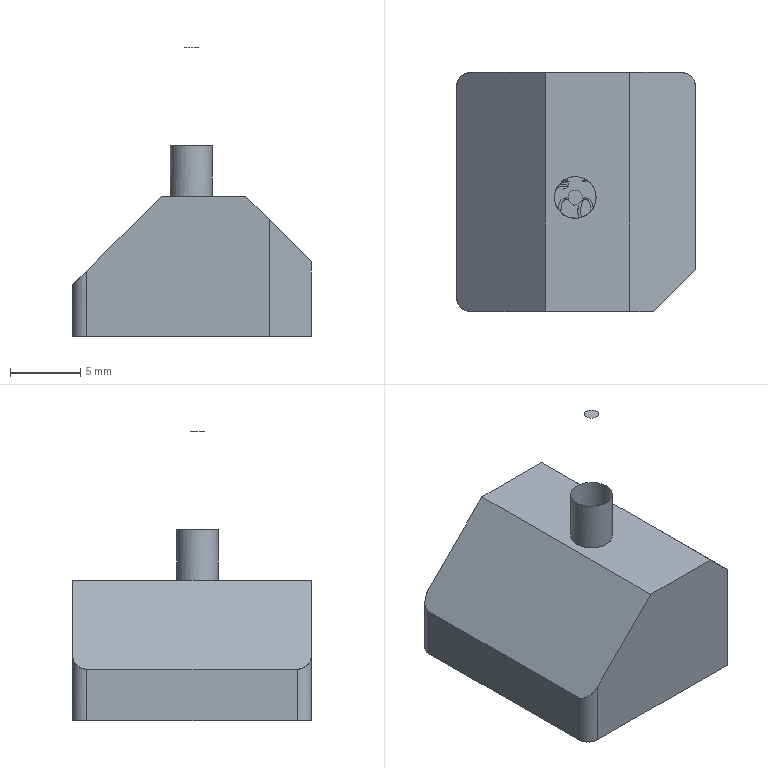NC program | PowerMill | posted with a generic post | part box 17 x 17 x 20.603 mm
Lines 1 to 1059 of 42778:
%
O0001
N104 ( POWERMILL CB  : 2026004.0)
N105 ( POST VER      : 2026.0.0.5161)
N106 ( OPTION FILE   : FANUC)
N107 ( OUTPUT WORKPLANE : WORLD)
N108 (  )
N109 ( TOOL LIST )
N110 (---------------------------------------)
N111 ( NO. | ID        | DIA.| TIP RAD|LENGTH)
N112 (---------------------------------------)
N113 (    1|D10C_1_1_1 |10.0 |  0.0   |76.04 )
N114 (    3|D10_1_1_1  |10.0 |  0.0   |75.76 )
N115 (   14|D4_2_1     | 4.0 |  0.0   |65.68 )
N116 (    7|R2_2_1     | 4.0 |  2.0   |73.16 )
N117 (   13|TEXT_D4_1_1| 4.0 |  0.3   |65.88 )
N118 (---------------------------------------)
N119 (  )
N120 ( NUMBER OF TOOLPATHS: 10.0 )
N121 ( ESTIMATED PROGRAM DURATION: 0 HOURS 5 MIN 41 SEC)
N122 (  )
N123 G00 G21 G80 G40 G17
N124 G90
N125 G54
N126 G53 Z0.0
N127 (---------------)
N128 ( START TOOLPATH : 粗公开粗01-扫面平行-D10C )
N129 (---------------)
N130 ( TOOL NO.    :1 )
N131 ( TOOL TYPE   : ENDMILL)
N132 ( TOOL ID     : D10C_1_1_1)
N133 ( TOOL DIA    : 10.0 LENGTH 76.04)
N134 T1
N135 M6
N136 S8000 M03
N137 G00 G90 X0.002 Y0.0
N138 G43 Z10.2 H1
N139
N140 G05 P10000 R4
N141 X16.202 Y11.2
N142 Z1.053
N143 G01 Z-0.147 F6000.0
N144 X11.202 F10000.0
N145 X-11.198
N146 Y5.6
N147 X11.202
N148 Y0.0
N149 X-11.198
N150 Y-5.6
N151 X11.202
N152 Y-11.2
N153 X-11.198
N154 X-16.198
N155 G00 Z10.2
N156 G05 P0
N157 (---------------)
N158 ( END TOOLPATH : 粗公开粗01-扫面平行-D10C )
N159 (---------------)
N160 ( START TOOLPATH : 粗公开粗01-外形偏置-D10C )
N161 (---------------)
N162 G00 X0.002 Y0.0 Z9.803
N163 G05 P10000 R4
N164 X5.2164 Y-16.475
N165 Z0.6159
N166 G01 Z-0.5841 F6000.0
N167 Y-15.9475 F10000.0
N168 G03 X0.4689 Y-11.2 I-4.7475 J0.0
N169 G01 X-10.198
N170 G02 X-11.198 Y-10.2 I0.0 J1.0
N171 G01 Y10.2
N172 G02 X-10.198 Y11.2 I1.0 J0.0
N173 G01 X10.202
N174 G02 X11.202 Y10.2 I0.0 J-1.0
N175 G01 Y-10.2
N176 G02 X10.202 Y-11.2 I-1.0 J0.0
N177 G01 X0.4689
N178 X0.3887 Y-6.1325
N179 X-0.3847 Y-6.1447
N180 X-1.1581 Y-6.0422
N181 X-1.9316 Y-5.8387
N182 X-2.705 Y-5.5007
N183 X-3.4724 Y-5.0273
N184 X-4.2518 Y-4.3313
N185 X-4.9075 Y-3.4804
N186 X-5.3237 Y-2.707
N187 X-5.5933 Y-1.9336
N188 X-5.7564 Y-1.1601
N189 X-5.8016 Y-0.3867
N190 X-5.7528 Y0.3867
N191 X-5.5859 Y1.1601
N192 X-5.3119 Y1.9336
N193 X-4.8907 Y2.707
N194 X-4.2993 Y3.4804
N195 X-3.4784 Y4.2225
N196 X-2.705 Y4.7005
N197 X-1.9645 Y5.0273
N198 X-1.1581 Y5.2423
N199 X-0.3847 Y5.3447
N200 X0.3887 Y5.3325
N201 X1.1621 Y5.2245
N202 X1.8447 Y5.0273
N203 X2.709 Y4.6479
N204 X3.4824 Y4.1366
N205 X4.1932 Y3.4804
N206 X4.7904 Y2.707
N207 X5.0293 Y2.2968
N208 X5.202 Y1.9336
N209 X5.4862 Y1.1601
N210 X5.6427 Y0.3867
N211 X5.702 Y-0.3867
N212 X5.6464 Y-1.1601
N213 X5.4936 Y-1.9336
N214 X5.2135 Y-2.707
N215 X5.0293 Y-3.0966
N216 X4.8073 Y-3.4804
N217 X4.2558 Y-4.2102
N218 X3.4824 Y-4.9368
N219 X2.709 Y-5.4482
N220 X1.9193 Y-5.8007
N221 X1.1621 Y-6.0245
N222 X0.3887 Y-6.1325
N223 X0.4689 Y-11.2
N224 G00 Z3.2287
N225 G01 X5.2164 Y-16.475
N226 G00 Z0.2287
N227 G01 Z-0.9713 F6000.0
N228 Y-15.9475 F10000.0
N229 G03 X0.4689 Y-11.2 I-4.7475 J0.0
N230 G01 X-10.198
N231 G02 X-11.198 Y-10.2 I0.0 J1.0
N232 G01 Y10.2
N233 G02 X-10.198 Y11.2 I1.0 J0.0
N234 G01 X10.202
N235 G02 X11.202 Y10.2 I0.0 J-1.0
N236 G01 Y-10.2
N237 G02 X10.202 Y-11.2 I-1.0 J0.0
N238 G01 X0.471
N239 X0.3887 Y-6.1865
N240 X-0.3847 Y-6.1992
N241 X-1.1581 Y-6.0972
N242 X-1.9316 Y-5.8961
N243 X-2.705 Y-5.5614
N244 X-3.4784 Y-5.0908
N245 X-4.2518 Y-4.4099
N246 X-4.3964 Y-4.2538
N247 X-4.9706 Y-3.4804
N248 X-5.3827 Y-2.707
N249 X-5.6493 Y-1.9336
N250 X-5.7987 Y-1.2475
N251 X-5.8555 Y-0.3867
N252 X-5.8077 Y0.3867
N253 X-5.6419 Y1.1601
N254 X-5.371 Y1.9336
N255 X-5.0253 Y2.5909
N256 X-4.3724 Y3.4804
N257 X-3.528 Y4.2538
N258 X-2.705 Y4.761
N259 X-2.1221 Y5.0273
N260 X-1.1581 Y5.2973
N261 X-0.3847 Y5.3992
N262 X0.3887 Y5.3865
N263 X1.1621 Y5.28
N264 X1.9356 Y5.0521
N265 X2.709 Y4.7095
N266 X3.4158 Y4.2538
N267 X4.2558 Y3.4915
N268 X4.8545 Y2.707
N269 X5.0293 Y2.4118
N270 X5.2607 Y1.9336
N271 X5.5424 Y1.1601
N272 X5.6972 Y0.3867
N273 X5.7564 Y-0.3867
N274 X5.7008 Y-1.1601
N275 X5.5498 Y-1.9336
N276 X5.2721 Y-2.707
N277 X5.0293 Y-3.2119
N278 X4.8713 Y-3.4804
N279 X4.2887 Y-4.2538
N280 X3.4824 Y-5.0044
N281 X2.709 Y-5.5102
N282 X2.0755 Y-5.8007
N283 X1.1621 Y-6.08
N284 X0.3887 Y-6.1865
N285 X0.471 Y-11.2
N286 X0.4689
N287 G00 Z2.8416
N288 G01 X5.2164 Y-16.475
N289 G00 Z-0.1584
N290 G01 Z-1.3584 F6000.0
N291 Y-15.9475 F10000.0
N292 G03 X0.4689 Y-11.2 I-4.7475 J0.0
N293 G01 X-10.198
N294 G02 X-11.198 Y-10.2 I0.0 J1.0
N295 G01 Y10.2
N296 G02 X-10.198 Y11.2 I1.0 J0.0
N297 G01 X10.202
N298 G02 X11.202 Y10.2 I0.0 J-1.0
N299 G01 Y-10.2
N300 G02 X10.202 Y-11.2 I-1.0 J0.0
N301 G01 X0.4729
N302 X0.3887 Y-6.2405
N303 X-0.3847 Y-6.2537
N304 X-1.1581 Y-6.1522
N305 X-1.9316 Y-5.9534
N306 X-2.3305 Y-5.8007
N307 X-2.705 Y-5.622
N308 X-3.4784 Y-5.1573
N309 X-4.2518 Y-4.4867
N310 X-4.4692 Y-4.2538
N311 X-5.0253 Y-3.4945
N312 X-5.4417 Y-2.707
N313 X-5.7052 Y-1.9336
N314 X-5.8661 Y-1.1601
N315 X-5.9094 Y-0.3867
N316 X-5.8626 Y0.3867
N317 X-5.6978 Y1.1601
N318 X-5.4302 Y1.9336
N319 X-5.0253 Y2.6939
N320 X-4.4456 Y3.4804
N321 X-4.2518 Y3.6874
N322 X-3.6168 Y4.2538
N323 X-2.705 Y4.8215
N324 X-2.2679 Y5.0273
N325 X-1.9316 Y5.1529
N326 X-1.1581 Y5.3523
N327 X-0.3847 Y5.4537
N328 X0.3887 Y5.4405
N329 X1.1621 Y5.3355
N330 X1.9356 Y5.1093
N331 X2.709 Y4.7711
N332 X3.5078 Y4.2538
N333 X4.2558 Y3.5736
N334 X4.9187 Y2.707
N335 X5.3193 Y1.9336
N336 X5.5987 Y1.1601
N337 X5.7516 Y0.3867
N338 X5.8108 Y-0.3867
N339 X5.7552 Y-1.1601
N340 X5.6059 Y-1.9336
N341 X5.3307 Y-2.707
N342 X4.9353 Y-3.4804
N343 X4.3605 Y-4.2538
N344 X3.5428 Y-5.0273
N345 X2.709 Y-5.5721
N346 X2.2229 Y-5.8007
N347 X1.9356 Y-5.9093
N348 X1.1621 Y-6.1355
N349 X0.3887 Y-6.2405
N350 X0.4729 Y-11.2
N351 X0.4689
N352 G00 Z2.4544
N353 G01 X5.2164 Y-16.475
N354 G00 Z-0.5456
N355 G01 Z-1.7456 F6000.0
N356 Y-15.9475 F10000.0
N357 G03 X0.4689 Y-11.2 I-4.7475 J0.0
N358 G01 X-10.198
N359 G02 X-11.198 Y-10.2 I0.0 J1.0
N360 G01 Y10.2
N361 G02 X-10.198 Y11.2 I1.0 J0.0
N362 G01 X10.202
N363 G02 X11.202 Y10.2 I0.0 J-1.0
N364 G01 Y-10.2
N365 G02 X10.202 Y-11.2 I-1.0 J0.0
N366 G01 X0.4748
N367 X0.3887 Y-6.2946
N368 X-0.3847 Y-6.3082
N369 X-1.1581 Y-6.2073
N370 X-1.9316 Y-6.0108
N371 X-2.705 Y-5.6827
N372 X-3.4784 Y-5.2239
N373 X-3.7387 Y-5.0273
N374 X-4.2518 Y-4.5626
N375 X-4.542 Y-4.2538
N376 X-5.0253 Y-3.5981
N377 X-5.5007 Y-2.707
N378 X-5.7612 Y-1.9336
N379 X-5.9209 Y-1.1601
N380 X-5.9633 Y-0.3867
N381 X-5.9174 Y0.3867
N382 X-5.7987 Y0.9956
N383 X-5.4893 Y1.9336
N384 X-5.0804 Y2.707
N385 X-4.5187 Y3.4804
N386 X-4.2518 Y3.7627
N387 X-3.7052 Y4.2538
N388 X-3.4784 Y4.4241
N389 X-2.705 Y4.882
N390 X-2.4058 Y5.0273
N391 X-1.9316 Y5.2101
N392 X-1.1581 Y5.4074
N393 X-0.3847 Y5.5082
N394 X0.3887 Y5.4946
N395 X1.1621 Y5.3909
N396 X1.9356 Y5.1665
N397 X2.3013 Y5.0273
N398 X2.709 Y4.8327
N399 X3.4824 Y4.3397
N400 X4.2558 Y3.6535
N401 X4.409 Y3.4804
N402 X4.9828 Y2.707
N403 X5.3779 Y1.9336
N404 X5.6549 Y1.1601
N405 X5.8027 Y0.4104
N406 X5.8652 Y-0.3867
N407 X5.8096 Y-1.1601
N408 X5.6621 Y-1.9336
N409 X5.3893 Y-2.707
N410 X5.0293 Y-3.4311
N411 X4.4315 Y-4.2538
N412 X4.2558 Y-4.4542
N413 X3.6311 Y-5.0273
N414 X2.709 Y-5.6333
N415 X2.3621 Y-5.8007
N416 X1.9356 Y-5.9665
N417 X1.1621 Y-6.1909
N418 X0.3887 Y-6.2946
N419 X0.4748 Y-11.2
N420 X0.4689
N421 G00 Z2.0673
N422 G01 X5.2164 Y-16.475
N423 G00 Z-0.9327
N424 G01 Z-2.1327 F6000.0
N425 Y-15.9475 F10000.0
N426 G03 X0.4689 Y-11.2 I-4.7475 J0.0
N427 G01 X-10.198
N428 G02 X-11.198 Y-10.2 I0.0 J1.0
N429 G01 Y10.2
N430 G02 X-10.198 Y11.2 I1.0 J0.0
N431 G01 X10.202
N432 G02 X11.202 Y10.2 I0.0 J-1.0
N433 G01 Y-10.2
N434 G02 X10.202 Y-11.2 I-1.0 J0.0
N435 G01 X0.4766
N436 X0.3887 Y-6.3486
N437 X-0.3847 Y-6.3626
N438 X-1.1581 Y-6.2623
N439 X-1.9316 Y-6.0682
N440 X-2.5905 Y-5.8007
N441 X-3.4784 Y-5.2904
N442 X-3.8234 Y-5.0273
N443 X-4.2518 Y-4.6386
N444 X-4.614 Y-4.2538
N445 X-5.0253 Y-3.6982
N446 X-5.16 Y-3.4804
N447 X-5.5597 Y-2.707
N448 X-5.7987 Y-1.9995
N449 X-5.9757 Y-1.1601
N450 X-6.0172 Y-0.3867
N451 X-5.9723 Y0.3867
N452 X-5.8098 Y1.1601
N453 X-5.5485 Y1.9336
N454 X-5.0253 Y2.8991
N455 X-4.5914 Y3.4804
N456 X-4.2518 Y3.838
N457 X-3.7915 Y4.2538
N458 X-3.4784 Y4.4913
N459 X-2.705 Y4.9424
N460 X-1.9316 Y5.2673
N461 X-1.1581 Y5.4624
N462 X-0.3847 Y5.5626
N463 X0.3887 Y5.5486
N464 X1.1621 Y5.4464
N465 X1.9356 Y5.2237
N466 X2.4369 Y5.0273
N467 X2.709 Y4.8943
N468 X3.4824 Y4.4056
N469 X3.6855 Y4.2538
N470 X4.2558 Y3.7327
N471 X4.4787 Y3.4804
N472 X5.0293 Y2.7365
N473 X5.4366 Y1.9336
N474 X5.7112 Y1.1601
N475 X5.8604 Y0.3867
N476 X5.9196 Y-0.3867
N477 X5.864 Y-1.1601
N478 X5.7182 Y-1.9336
N479 X5.4479 Y-2.707
N480 X5.0632 Y-3.4804
N481 X4.5011 Y-4.2538
N482 X4.2558 Y-4.5328
N483 X3.7194 Y-5.0273
N484 X3.4824 Y-5.2058
N485 X2.709 Y-5.6944
N486 X2.4942 Y-5.8007
N487 X1.9356 Y-6.0237
N488 X1.1621 Y-6.2464
N489 X0.3887 Y-6.3486
N490 X0.4766 Y-11.2
N491 X0.4689
N492 G00 Z1.6801
N493 G01 X5.2164 Y-16.475
N494 G00 Z-1.3199
N495 G01 Z-2.5199 F6000.0
N496 Y-15.9475 F10000.0
N497 G03 X0.4689 Y-11.2 I-4.7475 J0.0
N498 G01 X-10.198
N499 G02 X-11.198 Y-10.2 I0.0 J1.0
N500 G01 Y10.2
N501 G02 X-10.198 Y11.2 I1.0 J0.0
N502 G01 X10.202
N503 G02 X11.202 Y10.2 I0.0 J-1.0
N504 G01 Y-10.2
N505 G02 X10.202 Y-11.2 I-1.0 J0.0
N506 G01 X0.4784
N507 X0.3887 Y-6.4026
N508 X-0.3847 Y-6.4171
N509 X-1.1581 Y-6.3174
N510 X-1.9316 Y-6.1255
N511 X-2.705 Y-5.804
N512 X-3.4784 Y-5.357
N513 X-3.9081 Y-5.0273
N514 X-4.2518 Y-4.713
N515 X-4.6845 Y-4.2538
N516 X-5.0253 Y-3.7983
N517 X-5.2231 Y-3.4804
N518 X-5.6187 Y-2.707
N519 X-5.8731 Y-1.9336
N520 X-6.0305 Y-1.1601
N521 X-6.0711 Y-0.3867
N522 X-6.0271 Y0.3867
N523 X-5.8657 Y1.1601
N524 X-5.6076 Y1.9336
N525 X-5.2068 Y2.707
N526 X-5.0253 Y2.9972
N527 X-4.6623 Y3.4804
N528 X-4.2518 Y3.9134
N529 X-3.8762 Y4.2538
N530 X-3.4784 Y4.5573
N531 X-2.6589 Y5.0273
N532 X-1.9316 Y5.3245
N533 X-1.1581 Y5.5175
N534 X-0.3847 Y5.6171
N535 X0.3887 Y5.6026
N536 X1.1621 Y5.5019
N537 X1.9356 Y5.2809
N538 X2.5657 Y5.0273
N539 X3.4824 Y4.4716
N540 X3.7727 Y4.2538
N541 X4.2558 Y3.8119
N542 X4.5483 Y3.4804
N543 X5.0293 Y2.8384
N544 X5.4952 Y1.9336
N545 X5.7674 Y1.1601
N546 X5.9148 Y0.3867
N547 X5.974 Y-0.3867
N548 X5.9184 Y-1.1601
N549 X5.8027 Y-1.8233
N550 X5.5065 Y-2.707
N551 X5.1272 Y-3.4804
N552 X4.5706 Y-4.2538
N553 X4.2558 Y-4.6115
N554 X3.8053 Y-5.0273
N555 X3.4824 Y-5.2718
N556 X2.6205 Y-5.8007
N557 X1.9356 Y-6.0809
N558 X1.1621 Y-6.3019
N559 X0.3887 Y-6.4026
N560 X0.4784 Y-11.2
N561 X0.4689
N562 G00 Z1.293
N563 G01 X5.2164 Y-16.475
N564 G00 Z-1.707
N565 G01 Z-2.907 F6000.0
N566 Y-15.9475 F10000.0
N567 G03 X0.4689 Y-11.2 I-4.7475 J0.0
N568 G01 X-10.198
N569 G02 X-11.198 Y-10.2 I0.0 J1.0
N570 G01 Y10.2
N571 G02 X-10.198 Y11.2 I1.0 J0.0
N572 G01 X10.202
N573 G02 X11.202 Y10.2 I0.0 J-1.0
N574 G01 Y-10.2
N575 G02 X10.202 Y-11.2 I-1.0 J0.0
N576 G01 X0.4801
N577 X0.3887 Y-6.4567
N578 X-0.3847 Y-6.4716
N579 X-1.1581 Y-6.3724
N580 X-1.9316 Y-6.1827
N581 X-2.705 Y-5.8647
N582 X-3.4784 Y-5.4235
N583 X-3.9903 Y-5.0273
N584 X-4.2518 Y-4.7867
N585 X-4.7551 Y-4.2538
N586 X-5.0253 Y-3.8941
N587 X-5.2862 Y-3.4804
N588 X-5.6777 Y-2.707
N589 X-5.929 Y-1.9336
N590 X-6.0853 Y-1.1601
N591 X-6.1251 Y-0.3867
N592 X-6.0819 Y0.3867
N593 X-5.9217 Y1.1601
N594 X-5.6667 Y1.9336
N595 X-5.27 Y2.707
N596 X-5.0253 Y3.0951
N597 X-4.7331 Y3.4804
N598 X-4.2518 Y3.9871
N599 X-3.9604 Y4.2538
N600 X-3.4784 Y4.6227
N601 X-2.7775 Y5.0273
N602 X-1.9316 Y5.3817
N603 X-1.1581 Y5.5725
N604 X-0.3847 Y5.6716
N605 X0.3887 Y5.6567
N606 X1.1621 Y5.5574
N607 X1.9356 Y5.3381
N608 X2.709 Y5.0176
N609 X3.4824 Y4.5376
N610 X3.8582 Y4.2538
N611 X4.2558 Y3.8899
N612 X4.6179 Y3.4804
N613 X5.0293 Y2.9377
N614 X5.1743 Y2.707
N615 X5.5538 Y1.9336
N616 X5.8027 Y1.2403
N617 X5.9692 Y0.3867
N618 X6.0284 Y-0.3867
N619 X5.9729 Y-1.1601
N620 X5.8305 Y-1.9336
N621 X5.5651 Y-2.707
N622 X5.1897 Y-3.4804
N623 X5.0293 Y-3.738
N624 X4.6402 Y-4.2538
N625 X4.2558 Y-4.6901
N626 X3.8902 Y-5.0273
N627 X3.4824 Y-5.3378
N628 X2.742 Y-5.8007
N629 X1.9356 Y-6.1381
N630 X1.1621 Y-6.3573
N631 X0.3887 Y-6.4567
N632 X0.4801 Y-11.2
N633 X0.4689
N634 G00 Z0.9058
N635 G01 X5.2164 Y-16.475
N636 G00 Z-2.0942
N637 G01 Z-3.2942 F6000.0
N638 Y-15.9475 F10000.0
N639 G03 X0.4689 Y-11.2 I-4.7475 J0.0
N640 G01 X-10.198
N641 G02 X-11.198 Y-10.2 I0.0 J1.0
N642 G01 Y10.2
N643 G02 X-10.198 Y11.2 I1.0 J0.0
N644 G01 X10.202
N645 G02 X11.202 Y10.2 I0.0 J-1.0
N646 G01 Y-10.2
N647 G02 X10.202 Y-11.2 I-1.0 J0.0
N648 G01 X0.4818
N649 X0.3887 Y-6.5107
N650 X-0.3847 Y-6.526
N651 X-1.1581 Y-6.4275
N652 X-1.9316 Y-6.2394
N653 X-2.705 Y-5.9253
N654 X-3.4784 Y-5.4887
N655 X-4.0717 Y-5.0273
N656 X-4.8256 Y-4.2538
N657 X-5.0253 Y-3.9899
N658 X-5.3493 Y-3.4804
N659 X-5.7367 Y-2.707
N660 X-5.985 Y-1.9336
N661 X-6.14 Y-1.1601
N662 X-6.179 Y-0.3867
N663 X-6.1367 Y0.3867
N664 X-5.9777 Y1.1601
N665 X-5.7259 Y1.9336
N666 X-5.3332 Y2.707
N667 X-5.0253 Y3.1891
N668 X-4.8039 Y3.4804
N669 X-4.0418 Y4.2538
N670 X-3.4784 Y4.6881
N671 X-2.8948 Y5.0273
N672 X-1.9316 Y5.4389
N673 X-1.1581 Y5.6275
N674 X-0.3847 Y5.726
N675 X0.3887 Y5.7107
N676 X1.1621 Y5.6128
N677 X1.9356 Y5.3953
N678 X2.709 Y5.0782
N679 X3.4824 Y4.6035
N680 X3.9437 Y4.2538
N681 X4.2558 Y3.9665
N682 X4.6876 Y3.4804
N683 X5.0293 Y3.035
N684 X5.2369 Y2.707
N685 X5.6125 Y1.9336
N686 X5.8027 Y1.4305
N687 X5.8799 Y1.1601
N688 X6.0236 Y0.3867
N689 X6.0828 Y-0.3867
N690 X6.0273 Y-1.1601
N691 X5.8867 Y-1.9336
N692 X5.8027 Y-2.231
N693 X5.6237 Y-2.707
N694 X5.2522 Y-3.4804
N695 X5.0293 Y-3.8347
N696 X4.7097 Y-4.2538
N697 X4.2558 Y-4.7668
N698 X3.9751 Y-5.0273
N699 X3.4824 Y-5.4038
N700 X2.8575 Y-5.8007
N701 X1.9356 Y-6.1953
N702 X1.1621 Y-6.4128
N703 X0.3887 Y-6.5107
N704 X0.4818 Y-11.2
N705 X0.4689
N706 G00 Z0.5187
N707 G01 X5.2164 Y-16.475
N708 G00 Z-2.4813
N709 G01 Z-3.6813 F6000.0
N710 Y-15.9475 F10000.0
N711 G03 X0.4689 Y-11.2 I-4.7475 J0.0
N712 G01 X-10.198
N713 G02 X-11.198 Y-10.2 I0.0 J1.0
N714 G01 Y10.2
N715 G02 X-10.198 Y11.2 I1.0 J0.0
N716 G01 X10.202
N717 G02 X11.202 Y10.2 I0.0 J-1.0
N718 G01 Y-10.2
N719 G02 X10.202 Y-11.2 I-1.0 J0.0
N720 G01 X0.7886
N721 X0.2512 Y-6.5741
N722 X-0.3847 Y-6.5805
N723 X-1.1581 Y-6.4825
N724 X-1.9316 Y-6.2961
N725 X-2.705 Y-5.9853
N726 X-3.4784 Y-5.5535
N727 X-4.1525 Y-5.0273
N728 X-4.8957 Y-4.2538
N729 X-5.4124 Y-3.4804
N730 X-5.7955 Y-2.707
N731 X-6.0409 Y-1.9336
N732 X-6.1948 Y-1.1601
N733 X-6.2329 Y-0.3867
N734 X-6.1915 Y0.3867
N735 X-6.0336 Y1.1601
N736 X-5.785 Y1.9336
N737 X-5.3964 Y2.707
N738 X-4.8746 Y3.4804
N739 X-4.2518 Y4.1346
N740 X-3.4784 Y4.7535
N741 X-2.705 Y5.1843
N742 X-1.9316 Y5.4961
N743 X-1.1581 Y5.6826
N744 X-0.3847 Y5.7805
N745 X0.3887 Y5.7647
N746 X1.1621 Y5.6683
N747 X1.9356 Y5.4525
N748 X2.709 Y5.1385
N749 X2.9228 Y5.0273
N750 X3.4824 Y4.6695
N751 X4.0268 Y4.2538
N752 X4.2558 Y4.0431
N753 X4.7572 Y3.4804
N754 X5.0293 Y3.1291
N755 X5.2996 Y2.707
N756 X5.6711 Y1.9336
N757 X5.8027 Y1.6007
N758 X5.9361 Y1.1601
N759 X6.078 Y0.3867
N760 X6.1373 Y-0.3867
N761 X6.0817 Y-1.1601
N762 X5.9428 Y-1.9336
N763 X5.8027 Y-2.4008
N764 X5.6823 Y-2.707
N765 X5.3147 Y-3.4804
N766 X5.0293 Y-3.9294
N767 X4.7792 Y-4.2538
N768 X4.2558 Y-4.8429
N769 X4.0571 Y-5.0273
N770 X3.4824 Y-5.4699
N771 X2.9692 Y-5.8007
N772 X2.709 Y-5.9387
N773 X1.9356 Y-6.2525
N774 X1.1621 Y-6.4683
N775 X0.2512 Y-6.5741
N776 X0.7886 Y-11.2
N777 X0.4689
N778 G00 Z0.1315
N779 G01 X5.2164 Y-16.475
N780 G00 Z-2.8685
N781 G01 Z-4.0685 F6000.0
N782 Y-15.9475 F10000.0
N783 G03 X0.4689 Y-11.2 I-4.7475 J0.0
N784 G01 X-10.198
N785 G02 X-11.198 Y-10.2 I0.0 J1.0
N786 G01 Y10.2
N787 G02 X-10.198 Y11.2 I1.0 J0.0
N788 G01 X10.202
N789 G02 X11.202 Y10.2 I0.0 J-1.0
N790 G01 Y-10.2
N791 G02 X10.202 Y-11.2 I-1.0 J0.0
N792 G01 X0.4849
N793 X0.3887 Y-6.6188
N794 X-0.3847 Y-6.635
N795 X-0.9587 Y-6.5741
N796 X-1.9316 Y-6.3528
N797 X-2.705 Y-6.0453
N798 X-3.4784 Y-5.6182
N799 X-4.2315 Y-5.0273
N800 X-4.9641 Y-4.2538
N801 X-5.4755 Y-3.4804
N802 X-5.7987 Y-2.8419
N803 X-6.0969 Y-1.9336
N804 X-6.2496 Y-1.1601
N805 X-6.2868 Y-0.3867
N806 X-6.2464 Y0.3867
N807 X-6.0896 Y1.1601
N808 X-5.8431 Y1.9336
N809 X-5.4595 Y2.707
N810 X-5.0253 Y3.3739
N811 X-4.2518 Y4.2083
N812 X-3.4784 Y4.8189
N813 X-2.705 Y5.2448
N814 X-1.9316 Y5.5533
N815 X-1.1581 Y5.7376
N816 X-0.3847 Y5.835
N817 X0.3887 Y5.8188
N818 X1.1621 Y5.7238
N819 X1.9356 Y5.5097
N820 X2.709 Y5.1989
N821 X3.0322 Y5.0273
N822 X3.4824 Y4.7355
N823 X4.2558 Y4.1196
N824 X4.8268 Y3.4804
N825 X5.0293 Y3.2221
N826 X5.3622 Y2.707
N827 X5.7298 Y1.9336
N828 X5.9924 Y1.1601
N829 X6.1324 Y0.3867
N830 X6.1917 Y-0.3867
N831 X6.1361 Y-1.1601
N832 X5.999 Y-1.9336
N833 X5.8027 Y-2.5569
N834 X5.3772 Y-3.4804
N835 X5.0293 Y-4.022
N836 X4.2558 Y-4.9189
N837 X3.4824 Y-5.5359
N838 X3.0786 Y-5.8007
N839 X2.709 Y-5.9998
N840 X1.9356 Y-6.3097
N841 X1.1621 Y-6.5238
N842 X0.8646 Y-6.5741
N843 X0.3887 Y-6.6188
N844 X0.4849 Y-11.2
N845 X0.4689
N846 G00 Z-0.2556
N847 G01 X5.2164 Y-16.475
N848 G00 Z-3.2556
N849 G01 Z-4.4556 F6000.0
N850 Y-15.9475 F10000.0
N851 G03 X0.4689 Y-11.2 I-4.7475 J0.0
N852 G01 X-10.198
N853 G02 X-11.198 Y-10.2 I0.0 J1.0
N854 G01 Y10.2
N855 G02 X-10.198 Y11.2 I1.0 J0.0
N856 G01 X10.202
N857 G02 X11.202 Y10.2 I0.0 J-1.0
N858 G01 Y-10.2
N859 G02 X10.202 Y-11.2 I-1.0 J0.0
N860 G01 X0.4863
N861 X0.3887 Y-6.6728
N862 X-0.3847 Y-6.6895
N863 X-1.1581 Y-6.5926
N864 X-1.9316 Y-6.4095
N865 X-2.705 Y-6.1053
N866 X-3.4784 Y-5.683
N867 X-4.2518 Y-5.0814
N868 X-5.0253 Y-4.2641
N869 X-5.5379 Y-3.4804
N870 X-5.7987 Y-2.9779
N871 X-5.9115 Y-2.707
N872 X-6.1528 Y-1.9336
N873 X-6.3044 Y-1.1601
N874 X-6.3407 Y-0.3867
N875 X-6.3012 Y0.3867
N876 X-6.1456 Y1.1601
N877 X-5.9012 Y1.9336
N878 X-5.7987 Y2.178
N879 X-5.522 Y2.707
N880 X-5.0121 Y3.4804
N881 X-4.2518 Y4.282
N882 X-3.4784 Y4.8837
N883 X-2.705 Y5.3053
N884 X-1.9316 Y5.6105
N885 X-1.1166 Y5.8007
N886 X-0.3847 Y5.8895
N887 X0.3887 Y5.8728
N888 X1.0486 Y5.8007
N889 X1.9356 Y5.5668
N890 X2.709 Y5.2593
N891 X3.1391 Y5.0273
N892 X3.4824 Y4.8014
N893 X4.1915 Y4.2538
N894 X4.8965 Y3.4804
N895 X5.4249 Y2.707
N896 X5.8027 Y1.9027
N897 X6.0486 Y1.1601
N898 X6.1868 Y0.3867
N899 X6.2461 Y-0.3867
N900 X6.1905 Y-1.1601
N901 X6.0551 Y-1.9336
N902 X5.7995 Y-2.707
N903 X5.4397 Y-3.4804
N904 X5.0293 Y-4.1123
N905 X4.2558 Y-4.9942
N906 X3.4824 Y-5.6019
N907 X3.1825 Y-5.8007
N908 X2.709 Y-6.0601
N909 X1.9356 Y-6.3668
N910 X1.1929 Y-6.5741
N911 X0.3887 Y-6.6728
N912 X0.4863 Y-11.2
N913 X0.4689
N914 G00 Z-0.6428
N915 G01 X5.2164 Y-16.475
N916 G00 Z-3.6428
N917 G01 Z-4.8428 F6000.0
N918 Y-15.9475 F10000.0
N919 G03 X0.4689 Y-11.2 I-4.7475 J0.0
N920 G01 X-10.198
N921 G02 X-11.198 Y-10.2 I0.0 J1.0
N922 G01 Y10.2
N923 G02 X-10.198 Y11.2 I1.0 J0.0
N924 G01 X10.202
N925 G02 X11.202 Y10.2 I0.0 J-1.0
N926 G01 Y-10.2
N927 G02 X10.202 Y-11.2 I-1.0 J0.0
N928 G01 X0.4877
N929 X0.3887 Y-6.7268
N930 X-0.3847 Y-6.7439
N931 X-1.1581 Y-6.6476
N932 X-1.9316 Y-6.4662
N933 X-2.705 Y-6.1653
N934 X-3.3928 Y-5.8007
N935 X-4.2518 Y-5.1551
N936 X-5.0253 Y-4.3524
N937 X-5.6001 Y-3.4804
N938 X-5.7987 Y-3.1072
N939 X-5.9695 Y-2.707
N940 X-6.2088 Y-1.9336
N941 X-6.3592 Y-1.1601
N942 X-6.3946 Y-0.3867
N943 X-6.356 Y0.3867
N944 X-6.2015 Y1.1601
N945 X-5.9593 Y1.9336
N946 X-5.7987 Y2.3072
N947 X-5.5844 Y2.707
N948 X-5.0809 Y3.4804
N949 X-4.3604 Y4.2538
N950 X-3.4784 Y4.9474
N951 X-2.705 Y5.3657
N952 X-1.9316 Y5.6672
N953 X-1.385 Y5.8007
N954 X-0.3847 Y5.9439
N955 X0.3887 Y5.9268
N956 X1.1621 Y5.8347
N957 X1.9356 Y5.624
N958 X2.709 Y5.3197
N959 X3.243 Y5.0273
N960 X3.4824 Y4.8674
N961 X4.2558 Y4.2678
N962 X4.9661 Y3.4804
N963 X5.4875 Y2.707
N964 X5.8027 Y2.0392
N965 X6.1049 Y1.1601
N966 X6.2413 Y0.3867
N967 X6.3005 Y-0.3867
N968 X6.2449 Y-1.1601
N969 X6.1113 Y-1.9336
N970 X5.8581 Y-2.707
N971 X5.5022 Y-3.4804
N972 X5.0293 Y-4.2008
N973 X4.2995 Y-5.0273
N974 X3.2847 Y-5.8007
N975 X2.709 Y-6.1199
N976 X1.9356 Y-6.424
N977 X1.4392 Y-6.5741
N978 X1.1621 Y-6.6347
N979 X0.3887 Y-6.7268
N980 X0.4877 Y-11.2
N981 X0.4689
N982 G00 Z-1.0299
N983 G01 X5.2164 Y-16.475
N984 G00 Z-4.0299
N985 G01 Z-5.2299 F6000.0
N986 Y-15.9475 F10000.0
N987 G03 X0.4689 Y-11.2 I-4.7475 J0.0
N988 G01 X-10.198
N989 G02 X-11.198 Y-10.2 I0.0 J1.0
N990 G01 Y10.2
N991 G02 X-10.198 Y11.2 I1.0 J0.0
N992 G01 X10.202
N993 G02 X11.202 Y10.2 I0.0 J-1.0
N994 G01 Y-10.2
N995 G02 X10.202 Y-11.2 I-1.0 J0.0
N996 G01 X0.4891
N997 X0.3887 Y-6.7808
N998 X-0.3847 Y-6.7984
N999 X-1.1581 Y-6.7027
N1000 X-1.7502 Y-6.5741
N1001 X-2.705 Y-6.2253
N1002 X-3.4784 Y-5.8119
N1003 X-4.2518 Y-5.2288
N1004 X-5.0253 Y-4.4401
N1005 X-5.1695 Y-4.2538
N1006 X-5.7987 Y-3.2303
N1007 X-6.0274 Y-2.707
N1008 X-6.2647 Y-1.9336
N1009 X-6.414 Y-1.1601
N1010 X-6.4485 Y-0.3867
N1011 X-6.4108 Y0.3867
N1012 X-6.2575 Y1.1601
N1013 X-6.0174 Y1.9336
N1014 X-5.7987 Y2.4303
N1015 X-5.6469 Y2.707
N1016 X-5.1496 Y3.4804
N1017 X-5.0253 Y3.6394
N1018 X-4.2518 Y4.4288
N1019 X-3.4784 Y5.0111
N1020 X-2.705 Y5.4262
N1021 X-1.9316 Y5.7237
N1022 X-1.1581 Y5.9027
N1023 X-0.3847 Y5.9984
N1024 X0.3887 Y5.9808
N1025 X1.1621 Y5.8902
N1026 X1.554 Y5.8007
N1027 X1.9356 Y5.6812
N1028 X2.709 Y5.38
N1029 X3.3429 Y5.0273
N1030 X4.2558 Y4.3419
N1031 X5.0293 Y3.4883
N1032 X5.5496 Y2.707
N1033 X5.9057 Y1.9336
N1034 X6.1611 Y1.1601
N1035 X6.2957 Y0.3867
N1036 X6.3549 Y-0.3867
N1037 X6.2993 Y-1.1601
N1038 X6.1674 Y-1.9336
N1039 X5.9167 Y-2.707
N1040 X5.5637 Y-3.4804
N1041 X5.0566 Y-4.2538
N1042 X4.3785 Y-5.0273
N1043 X3.4824 Y-5.7329
N1044 X2.709 Y-6.1798
N1045 X1.6487 Y-6.5741
N1046 X1.1621 Y-6.6902
N1047 X0.3887 Y-6.7808
N1048 X0.4891 Y-11.2
N1049 X0.4689
N1050 G00 Z-1.4171
N1051 G01 X5.2164 Y-16.475
N1052 G00 Z-4.4171
N1053 G01 Z-5.6171 F6000.0
N1054 Y-15.9475 F10000.0
N1055 G03 X0.4689 Y-11.2 I-4.7475 J0.0
N1056 G01 X-10.198
N1057 G02 X-11.198 Y-10.2 I0.0 J1.0
N1058 G01 Y10.2
N1059 G02 X-10.198 Y11.2 I1.0 J0.0
N1060 G01 X10.202
N1061 G02 X11.202 Y10.2 I0.0 J-1.0
N1062 G01 Y-10.2
N1063 G02 X10.202 Y-11.2 I-1.0 J0.0
N1064 G01 X0.4903
N1065 X0.3887 Y-6.8349
N1066 X-0.3847 Y-6.8529
N1067 X-1.1581 Y-6.7577
N1068 X-1.9536 Y-6.5741
N1069 X-2.705 Y-6.2853
N1070 X-3.4784 Y-5.875
N1071 X-4.2518 Y-5.3016
N1072 X-4.5475 Y-5.0273
N1073 X-5.0253 Y-4.5249
N1074 X-5.2367 Y-4.2538
N1075 X-5.7247 Y-3.4804
N1076 X-6.0854 Y-2.707
N1077 X-6.3207 Y-1.9336
N1078 X-6.4687 Y-1.1601
N1079 X-6.5024 Y-0.3867
N1080 X-6.4657 Y0.3867
N1081 X-6.3135 Y1.1601
N1082 X-6.0756 Y1.9336
N1083 X-5.7987 Y2.5475
N1084 X-5.2173 Y3.4804
N1085 X-5.0253 Y3.7257
N1086 X-4.2518 Y4.501
N1087 X-3.5568 Y5.0273
N1088 X-2.705 Y5.4863
N1089 X-1.9316 Y5.7803
N1090 X-1.1581 Y5.9578
N1091 X-0.3847 Y6.0529
N1092 X0.3887 Y6.0349
N1093 X1.1621 Y5.9456
N1094 X1.7486 Y5.8007
N1095 X2.709 Y5.4404
N1096 X3.4416 Y5.0273
N1097 X4.2558 Y4.4149
N1098 X4.4301 Y4.2538
N1099 X5.0293 Y3.5738
N1100 X5.6109 Y2.707
N1101 X5.9643 Y1.9336
N1102 X6.2174 Y1.1601
N1103 X6.3501 Y0.3867
N1104 X6.4093 Y-0.3867
N1105 X6.3537 Y-1.1601
N1106 X6.2236 Y-1.9336
N1107 X5.9753 Y-2.707
N1108 X5.6249 Y-3.4804
N1109 X5.1248 Y-4.2538
N1110 X4.4571 Y-5.0273
N1111 X4.2558 Y-5.2151
N1112 X3.4804 Y-5.8007
N1113 X2.709 Y-6.2396
N1114 X1.8305 Y-6.5741
N1115 X1.1621 Y-6.7456
N1116 X0.3887 Y-6.8349
N1117 X0.4903 Y-11.2
N1118 X0.4689
N1119 G00 Z-1.8042
N1120 G01 X5.2164 Y-16.475
N1121 G00 Z-4.8042
N1122 G01 Z-6.0042 F6000.0
N1123 Y-15.9475 F10000.0
N1124 G03 X0.4689 Y-11.2 I-4.7475 J0.0
N1125 G01 X-10.198
N1126 G02 X-11.198 Y-10.2 I0.0 J1.0
N1127 G01 Y10.2
N1128 G02 X-10.198 Y11.2 I1.0 J0.0
N1129 G01 X10.202
N1130 G02 X11.202 Y10.2 I0.0 J-1.0
N1131 G01 Y-10.2
N1132 G02 X10.202 Y-11.2 I-1.0 J0.0
N1133 G01 X0.4915
N1134 X0.3887 Y-6.8889
N1135 X-0.3847 Y-6.9073
N1136 X-1.1581 Y-6.8128
N1137 X-1.9316 Y-6.6363
N1138 X-2.705 Y-6.3453
N1139 X-3.4784 Y-5.9381
N1140 X-3.6964 Y-5.8007
N1141 X-4.2518 Y-5.3734
N1142 X-4.6256 Y-5.0273
N1143 X-5.0253 Y-4.6098
N1144 X-5.3031 Y-4.2538
N1145 X-5.7987 Y-3.4603
N1146 X-6.1434 Y-2.707
N1147 X-6.3766 Y-1.9336
N1148 X-6.5235 Y-1.1601
N1149 X-6.5563 Y-0.3867
N1150 X-6.5205 Y0.3867
N1151 X-6.3694 Y1.1601
N1152 X-6.1337 Y1.9336
N1153 X-5.7987 Y2.6603
N1154 X-5.2841 Y3.4804
N1155 X-5.0253 Y3.8092
N1156 X-4.5967 Y4.2538